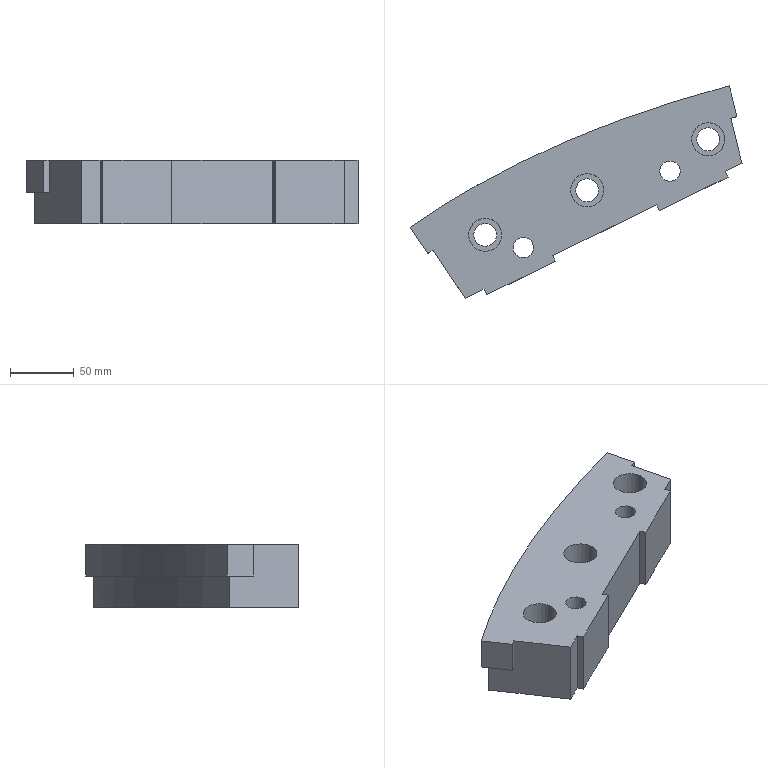Part | NX | features solid 2 | 1 solid | 31 faces | box 260.567 x 166.598 x 50 mm | volume 838150 mm3 | plane 19 | cylinder 8 | spline 4 | commonest cylinder face diameters 18 x3 26 x3 16 x2
STEP:
#1=CARTESIAN_POINT('',(-498.047,350.703,-50.));
#2=VERTEX_POINT('',#1);
#3=CARTESIAN_POINT('',(-507.047,350.703,-50.));
#4=DIRECTION('',(0.,0.,1.));
#5=DIRECTION('',(1.,0.,0.));
#6=AXIS2_PLACEMENT_3D('',#3,#4,#5);
#7=CIRCLE('',#6,9.);
#8=EDGE_CURVE('',#2,#2,#7,.T.);
#9=ORIENTED_EDGE('',*,*,#8,.T.);
#10=EDGE_LOOP('',(#9));
#11=FACE_BOUND('',#10,.T.);
#12=CARTESIAN_POINT('',(-469.047,340.703,-50.));
#13=VERTEX_POINT('',#12);
#14=CARTESIAN_POINT('',(-477.047,340.703,-50.));
#15=DIRECTION('',(0.,0.,1.));
#16=DIRECTION('',(1.,0.,0.));
#17=AXIS2_PLACEMENT_3D('',#14,#15,#16);
#18=CIRCLE('',#17,8.);
#19=EDGE_CURVE('',#13,#13,#18,.T.);
#20=ORIENTED_EDGE('',*,*,#19,.T.);
#21=EDGE_LOOP('',(#20));
#22=FACE_BOUND('',#21,.T.);
#23=CARTESIAN_POINT('',(-354.047,400.703,-50.));
#24=VERTEX_POINT('',#23);
#25=CARTESIAN_POINT('',(-362.047,400.703,-50.));
#26=DIRECTION('',(0.,0.,1.));
#27=DIRECTION('',(1.,0.,0.));
#28=AXIS2_PLACEMENT_3D('',#25,#26,#27);
#29=CIRCLE('',#28,8.);
#30=EDGE_CURVE('',#24,#24,#29,.T.);
#31=ORIENTED_EDGE('',*,*,#30,.T.);
#32=EDGE_LOOP('',(#31));
#33=FACE_BOUND('',#32,.T.);
#34=CARTESIAN_POINT('',(-323.047,425.703,-50.));
#35=VERTEX_POINT('',#34);
#36=CARTESIAN_POINT('',(-332.047,425.703,-50.));
#37=DIRECTION('',(0.,0.,1.));
#38=DIRECTION('',(1.,0.,0.));
#39=AXIS2_PLACEMENT_3D('',#36,#37,#38);
#40=CIRCLE('',#39,9.);
#41=EDGE_CURVE('',#35,#35,#40,.T.);
#42=ORIENTED_EDGE('',*,*,#41,.T.);
#43=EDGE_LOOP('',(#42));
#44=FACE_BOUND('',#43,.T.);
#45=CARTESIAN_POINT('',(-522.586,301.062,-50.));
#46=VERTEX_POINT('',#45);
#47=CARTESIAN_POINT('',(-508.006,308.173,-50.));
#48=VERTEX_POINT('',#47);
#49=CARTESIAN_POINT('',(-578.443,273.819,-50.));
#50=DIRECTION('',(0.8988,0.4384,0.));
#51=VECTOR('',#50,1000.);
#52=LINE('',#49,#51);
#53=EDGE_CURVE('',#46,#48,#52,.T.);
#54=ORIENTED_EDGE('',*,*,#53,.F.);
#55=CARTESIAN_POINT('',(-559.181,355.316,-50.));
#56=VERTEX_POINT('',#55);
#57=CARTESIAN_POINT('',(158.716,-709.011,-50.));
#58=DIRECTION('',(-0.5592,0.829,0.));
#59=VECTOR('',#58,1000.);
#60=LINE('',#57,#59);
#61=EDGE_CURVE('',#46,#56,#60,.T.);
#62=ORIENTED_EDGE('',*,*,#61,.T.);
#63=CARTESIAN_POINT('',(-319.133,461.526,-50.));
#64=VERTEX_POINT('',#63);
#65=CARTESIAN_POINT('',(-559.181,355.316,-50.));
#66=CARTESIAN_POINT('',(-554.765,358.346,-50.));
#67=CARTESIAN_POINT('',(-545.797,364.324,-50.));
#68=CARTESIAN_POINT('',(-531.933,373.042,-50.));
#69=CARTESIAN_POINT('',(-520.049,380.094,-50.));
#70=CARTESIAN_POINT('',(-511.534,384.931,-50.));
#71=CARTESIAN_POINT('',(-506.645,387.648,-50.));
#72=CARTESIAN_POINT('',(-502.873,389.713,-50.));
#73=CARTESIAN_POINT('',(-499.379,391.6,-50.));
#74=CARTESIAN_POINT('',(-494.59,394.15,-50.));
#75=CARTESIAN_POINT('',(-486.188,398.533,-50.));
#76=CARTESIAN_POINT('',(-473.957,404.65,-50.));
#77=CARTESIAN_POINT('',(-461.477,410.549,-50.));
#78=CARTESIAN_POINT('',(-452.581,414.577,-50.));
#79=CARTESIAN_POINT('',(-447.486,416.835,-50.));
#80=CARTESIAN_POINT('',(-443.565,418.547,-50.));
#81=CARTESIAN_POINT('',(-439.928,420.112,-50.));
#82=CARTESIAN_POINT('',(-434.948,422.227,-50.));
#83=CARTESIAN_POINT('',(-426.215,425.856,-50.));
#84=CARTESIAN_POINT('',(-413.532,430.907,-50.));
#85=CARTESIAN_POINT('',(-400.591,435.769,-50.));
#86=CARTESIAN_POINT('',(-390.125,439.533,-50.));
#87=CARTESIAN_POINT('',(-382.095,442.334,-50.));
#88=CARTESIAN_POINT('',(-374.392,444.943,-50.));
#89=CARTESIAN_POINT('',(-363.96,448.377,-50.));
#90=CARTESIAN_POINT('',(-345.662,454.133,-50.));
#91=CARTESIAN_POINT('',(-329.787,458.676,-50.));
#92=CARTESIAN_POINT('',(-319.133,461.526,-50.));
#93=B_SPLINE_CURVE_WITH_KNOTS('',3,(#65,#66,#67,#68,#69,#70,#71,#72,#73,#74,#75,#76,#77,#78,#79,#80,#81,#82,#83,#84,#85,#86,#87,#88,#89,#90,#91,#92),.UNSPECIFIED.,.F.,.F.,(4,1,1,1,1,1,1,1,1,1,1,1,1,1,1,1,1,1,1,1,1,1,1,1,1,4),(0.,0.0625,0.125,0.1875,0.2188,0.2344,0.25,0.2656,0.2812,0.3125,0.375,0.4375,0.4688,0.4844,0.5,0.5156,0.5312,0.5625,0.625,0.6875,0.7188,0.75,0.7812,0.8125,0.875,1.),.UNSPECIFIED.);
#94=EDGE_CURVE('',#56,#64,#93,.T.);
#95=ORIENTED_EDGE('',*,*,#94,.T.);
#96=CARTESIAN_POINT('',(-305.521,406.931,-50.));
#97=VERTEX_POINT('',#96);
#98=CARTESIAN_POINT('',(2.961,-830.323,-50.));
#99=DIRECTION('',(-0.2419,0.9703,0.));
#100=VECTOR('',#99,1000.);
#101=LINE('',#98,#100);
#102=EDGE_CURVE('',#97,#64,#101,.T.);
#103=ORIENTED_EDGE('',*,*,#102,.F.);
#104=CARTESIAN_POINT('',(-318.612,400.547,-50.));
#105=VERTEX_POINT('',#104);
#106=CARTESIAN_POINT('',(-578.443,273.819,-50.));
#107=DIRECTION('',(0.8988,0.4384,0.));
#108=VECTOR('',#107,1000.);
#109=LINE('',#106,#108);
#110=EDGE_CURVE('',#105,#97,#109,.T.);
#111=ORIENTED_EDGE('',*,*,#110,.F.);
#112=CARTESIAN_POINT('',(-316.42,396.053,-50.));
#113=VERTEX_POINT('',#112);
#114=CARTESIAN_POINT('',(-309.844,382.571,-50.));
#115=DIRECTION('',(0.4384,-0.8988,0.));
#116=VECTOR('',#115,1000.);
#117=LINE('',#114,#116);
#118=EDGE_CURVE('',#105,#113,#117,.T.);
#119=ORIENTED_EDGE('',*,*,#118,.T.);
#120=CARTESIAN_POINT('',(-370.348,369.75,-50.));
#121=VERTEX_POINT('',#120);
#122=CARTESIAN_POINT('',(-576.251,269.325,-50.));
#123=DIRECTION('',(0.8988,0.4384,0.));
#124=VECTOR('',#123,1000.);
#125=LINE('',#122,#124);
#126=EDGE_CURVE('',#121,#113,#125,.T.);
#127=ORIENTED_EDGE('',*,*,#126,.F.);
#128=CARTESIAN_POINT('',(-372.54,374.244,-50.));
#129=VERTEX_POINT('',#128);
#130=CARTESIAN_POINT('',(-363.772,356.268,-50.));
#131=DIRECTION('',(0.4384,-0.8988,0.));
#132=VECTOR('',#131,1000.);
#133=LINE('',#130,#132);
#134=EDGE_CURVE('',#129,#121,#133,.T.);
#135=ORIENTED_EDGE('',*,*,#134,.F.);
#136=CARTESIAN_POINT('',(-454.078,334.475,-50.));
#137=VERTEX_POINT('',#136);
#138=CARTESIAN_POINT('',(-578.443,273.819,-50.));
#139=DIRECTION('',(0.8988,0.4384,0.));
#140=VECTOR('',#139,1000.);
#141=LINE('',#138,#140);
#142=EDGE_CURVE('',#137,#129,#141,.T.);
#143=ORIENTED_EDGE('',*,*,#142,.F.);
#144=CARTESIAN_POINT('',(-451.886,329.981,-50.));
#145=VERTEX_POINT('',#144);
#146=CARTESIAN_POINT('',(-445.311,316.499,-50.));
#147=DIRECTION('',(0.4384,-0.8988,0.));
#148=VECTOR('',#147,1000.);
#149=LINE('',#146,#148);
#150=EDGE_CURVE('',#137,#145,#149,.T.);
#151=ORIENTED_EDGE('',*,*,#150,.T.);
#152=CARTESIAN_POINT('',(-505.814,303.679,-50.));
#153=VERTEX_POINT('',#152);
#154=CARTESIAN_POINT('',(-576.251,269.325,-50.));
#155=DIRECTION('',(0.8988,0.4384,0.));
#156=VECTOR('',#155,1000.);
#157=LINE('',#154,#156);
#158=EDGE_CURVE('',#153,#145,#157,.T.);
#159=ORIENTED_EDGE('',*,*,#158,.F.);
#160=CARTESIAN_POINT('',(-499.239,290.197,-50.));
#161=DIRECTION('',(0.4384,-0.8988,0.));
#162=VECTOR('',#161,1000.);
#163=LINE('',#160,#162);
#164=EDGE_CURVE('',#48,#153,#163,.T.);
#165=ORIENTED_EDGE('',*,*,#164,.F.);
#166=EDGE_LOOP('',(#54,#62,#95,#103,#111,#119,#127,#135,#143,#151,#159,#165));
#167=FACE_BOUND('',#166,.T.);
#168=CARTESIAN_POINT('',(-418.047,385.703,-50.));
#169=VERTEX_POINT('',#168);
#170=CARTESIAN_POINT('',(-427.047,385.703,-50.));
#171=DIRECTION('',(0.,0.,1.));
#172=DIRECTION('',(1.,0.,0.));
#173=AXIS2_PLACEMENT_3D('',#170,#171,#172);
#174=CIRCLE('',#173,9.);
#175=EDGE_CURVE('',#169,#169,#174,.F.);
#176=ORIENTED_EDGE('',*,*,#175,.F.);
#177=EDGE_LOOP('',(#176));
#178=FACE_BOUND('',#177,.T.);
#179=CARTESIAN_POINT('',(-35.268,-839.855,-50.));
#180=DIRECTION('',(0.,0.,1.));
#181=DIRECTION('',(1.,0.,0.));
#182=AXIS2_PLACEMENT_3D('',#179,#180,#181);
#183=PLANE('',#182);
#184=ADVANCED_FACE('',(#11,#22,#33,#44,#167,#178),#183,.F.);
#185=CARTESIAN_POINT('',(-414.047,385.703,-30.));
#186=VERTEX_POINT('',#185);
#187=CARTESIAN_POINT('',(-427.047,385.703,-30.));
#188=DIRECTION('',(0.,0.,1.));
#189=DIRECTION('',(1.,0.,0.));
#190=AXIS2_PLACEMENT_3D('',#187,#188,#189);
#191=CIRCLE('',#190,13.);
#192=EDGE_CURVE('',#186,#186,#191,.T.);
#193=ORIENTED_EDGE('',*,*,#192,.T.);
#194=EDGE_LOOP('',(#193));
#195=FACE_BOUND('',#194,.T.);
#196=CARTESIAN_POINT('',(-418.047,385.703,-30.));
#197=VERTEX_POINT('',#196);
#198=CARTESIAN_POINT('',(-427.047,385.703,-30.));
#199=DIRECTION('',(0.,0.,1.));
#200=DIRECTION('',(1.,0.,0.));
#201=AXIS2_PLACEMENT_3D('',#198,#199,#200);
#202=CIRCLE('',#201,9.);
#203=EDGE_CURVE('',#197,#197,#202,.F.);
#204=ORIENTED_EDGE('',*,*,#203,.T.);
#205=EDGE_LOOP('',(#204));
#206=FACE_BOUND('',#205,.T.);
#207=CARTESIAN_POINT('',(-427.047,385.703,-30.));
#208=DIRECTION('',(0.,0.,1.));
#209=DIRECTION('',(1.,0.,0.));
#210=AXIS2_PLACEMENT_3D('',#207,#208,#209);
#211=PLANE('',#210);
#212=ADVANCED_FACE('',(#195,#206),#211,.T.);
#213=CARTESIAN_POINT('',(-354.047,400.703,0.));
#214=VERTEX_POINT('',#213);
#215=CARTESIAN_POINT('',(-362.047,400.703,0.));
#216=DIRECTION('',(0.,0.,1.));
#217=DIRECTION('',(1.,0.,0.));
#218=AXIS2_PLACEMENT_3D('',#215,#216,#217);
#219=CIRCLE('',#218,8.);
#220=EDGE_CURVE('',#214,#214,#219,.T.);
#221=ORIENTED_EDGE('',*,*,#220,.F.);
#222=EDGE_LOOP('',(#221));
#223=FACE_BOUND('',#222,.T.);
#224=CARTESIAN_POINT('',(-469.047,340.703,0.));
#225=VERTEX_POINT('',#224);
#226=CARTESIAN_POINT('',(-477.047,340.703,0.));
#227=DIRECTION('',(0.,0.,1.));
#228=DIRECTION('',(1.,0.,0.));
#229=AXIS2_PLACEMENT_3D('',#226,#227,#228);
#230=CIRCLE('',#229,8.);
#231=EDGE_CURVE('',#225,#225,#230,.T.);
#232=ORIENTED_EDGE('',*,*,#231,.F.);
#233=EDGE_LOOP('',(#232));
#234=FACE_BOUND('',#233,.T.);
#235=CARTESIAN_POINT('',(-319.047,425.703,0.));
#236=VERTEX_POINT('',#235);
#237=CARTESIAN_POINT('',(-332.047,425.703,0.));
#238=DIRECTION('',(0.,0.,1.));
#239=DIRECTION('',(1.,0.,0.));
#240=AXIS2_PLACEMENT_3D('',#237,#238,#239);
#241=CIRCLE('',#240,13.);
#242=EDGE_CURVE('',#236,#236,#241,.T.);
#243=ORIENTED_EDGE('',*,*,#242,.F.);
#244=EDGE_LOOP('',(#243));
#245=FACE_BOUND('',#244,.T.);
#246=CARTESIAN_POINT('',(-494.047,350.703,0.));
#247=VERTEX_POINT('',#246);
#248=CARTESIAN_POINT('',(-507.047,350.703,0.));
#249=DIRECTION('',(0.,0.,1.));
#250=DIRECTION('',(1.,0.,0.));
#251=AXIS2_PLACEMENT_3D('',#248,#249,#250);
#252=CIRCLE('',#251,13.);
#253=EDGE_CURVE('',#247,#247,#252,.T.);
#254=ORIENTED_EDGE('',*,*,#253,.F.);
#255=EDGE_LOOP('',(#254));
#256=FACE_BOUND('',#255,.T.);
#257=CARTESIAN_POINT('',(-552.106,335.886,0.));
#258=VERTEX_POINT('',#257);
#259=CARTESIAN_POINT('',(-566.088,356.614,0.));
#260=VERTEX_POINT('',#259);
#261=CARTESIAN_POINT('',(-500.019,258.663,0.));
#262=DIRECTION('',(-0.5592,0.829,0.));
#263=VECTOR('',#262,1000.);
#264=LINE('',#261,#263);
#265=EDGE_CURVE('',#258,#260,#264,.T.);
#266=ORIENTED_EDGE('',*,*,#265,.F.);
#267=CARTESIAN_POINT('',(-547.997,338.734,0.));
#268=VERTEX_POINT('',#267);
#269=CARTESIAN_POINT('',(-547.997,338.734,0.));
#270=CARTESIAN_POINT('',(-549.371,337.791,0.));
#271=CARTESIAN_POINT('',(-550.74,336.84,0.));
#272=CARTESIAN_POINT('',(-552.106,335.886,0.));
#273=B_SPLINE_CURVE_WITH_KNOTS('',3,(#269,#270,#271,#272),.UNSPECIFIED.,.F.,.F.,(4,4),(0.5979,0.6029),.UNSPECIFIED.);
#274=EDGE_CURVE('',#258,#268,#273,.F.);
#275=ORIENTED_EDGE('',*,*,#274,.T.);
#276=CARTESIAN_POINT('',(-522.586,301.062,0.));
#277=VERTEX_POINT('',#276);
#278=CARTESIAN_POINT('',(-497.568,263.971,0.));
#279=DIRECTION('',(0.5592,-0.829,0.));
#280=VECTOR('',#279,1000.);
#281=LINE('',#278,#280);
#282=EDGE_CURVE('',#268,#277,#281,.T.);
#283=ORIENTED_EDGE('',*,*,#282,.T.);
#284=CARTESIAN_POINT('',(-508.006,308.173,0.));
#285=VERTEX_POINT('',#284);
#286=CARTESIAN_POINT('',(-521.061,301.806,0.));
#287=DIRECTION('',(-0.8988,-0.4384,0.));
#288=VECTOR('',#287,1000.);
#289=LINE('',#286,#288);
#290=EDGE_CURVE('',#285,#277,#289,.T.);
#291=ORIENTED_EDGE('',*,*,#290,.F.);
#292=CARTESIAN_POINT('',(-505.814,303.679,0.));
#293=VERTEX_POINT('',#292);
#294=CARTESIAN_POINT('',(-538.254,370.19,0.));
#295=DIRECTION('',(0.4384,-0.8988,0.));
#296=VECTOR('',#295,1000.);
#297=LINE('',#294,#296);
#298=EDGE_CURVE('',#285,#293,#297,.T.);
#299=ORIENTED_EDGE('',*,*,#298,.T.);
#300=CARTESIAN_POINT('',(-451.886,329.981,0.));
#301=VERTEX_POINT('',#300);
#302=CARTESIAN_POINT('',(-518.869,297.312,0.));
#303=DIRECTION('',(0.8988,0.4384,0.));
#304=VECTOR('',#303,1000.);
#305=LINE('',#302,#304);
#306=EDGE_CURVE('',#293,#301,#305,.T.);
#307=ORIENTED_EDGE('',*,*,#306,.T.);
#308=CARTESIAN_POINT('',(-454.078,334.475,0.));
#309=VERTEX_POINT('',#308);
#310=CARTESIAN_POINT('',(-484.326,396.492,0.));
#311=DIRECTION('',(0.4384,-0.8988,0.));
#312=VECTOR('',#311,1000.);
#313=LINE('',#310,#312);
#314=EDGE_CURVE('',#309,#301,#313,.T.);
#315=ORIENTED_EDGE('',*,*,#314,.F.);
#316=CARTESIAN_POINT('',(-372.54,374.244,0.));
#317=VERTEX_POINT('',#316);
#318=CARTESIAN_POINT('',(-521.061,301.806,0.));
#319=DIRECTION('',(-0.8988,-0.4384,0.));
#320=VECTOR('',#319,1000.);
#321=LINE('',#318,#320);
#322=EDGE_CURVE('',#317,#309,#321,.T.);
#323=ORIENTED_EDGE('',*,*,#322,.F.);
#324=CARTESIAN_POINT('',(-370.348,369.75,0.));
#325=VERTEX_POINT('',#324);
#326=CARTESIAN_POINT('',(-402.787,436.261,0.));
#327=DIRECTION('',(0.4384,-0.8988,0.));
#328=VECTOR('',#327,1000.);
#329=LINE('',#326,#328);
#330=EDGE_CURVE('',#317,#325,#329,.T.);
#331=ORIENTED_EDGE('',*,*,#330,.T.);
#332=CARTESIAN_POINT('',(-316.42,396.053,0.));
#333=VERTEX_POINT('',#332);
#334=CARTESIAN_POINT('',(-518.869,297.312,0.));
#335=DIRECTION('',(0.8988,0.4384,0.));
#336=VECTOR('',#335,1000.);
#337=LINE('',#334,#336);
#338=EDGE_CURVE('',#325,#333,#337,.T.);
#339=ORIENTED_EDGE('',*,*,#338,.T.);
#340=CARTESIAN_POINT('',(-318.612,400.547,0.));
#341=VERTEX_POINT('',#340);
#342=CARTESIAN_POINT('',(-348.86,462.564,0.));
#343=DIRECTION('',(0.4384,-0.8988,0.));
#344=VECTOR('',#343,1000.);
#345=LINE('',#342,#344);
#346=EDGE_CURVE('',#341,#333,#345,.T.);
#347=ORIENTED_EDGE('',*,*,#346,.F.);
#348=CARTESIAN_POINT('',(-305.521,406.931,0.));
#349=VERTEX_POINT('',#348);
#350=CARTESIAN_POINT('',(-521.061,301.806,0.));
#351=DIRECTION('',(-0.8988,-0.4384,0.));
#352=VECTOR('',#351,1000.);
#353=LINE('',#350,#352);
#354=EDGE_CURVE('',#349,#341,#353,.T.);
#355=ORIENTED_EDGE('',*,*,#354,.F.);
#356=CARTESIAN_POINT('',(-314.294,442.117,0.));
#357=VERTEX_POINT('',#356);
#358=CARTESIAN_POINT('',(-294.648,363.324,0.));
#359=DIRECTION('',(0.2419,-0.9703,0.));
#360=VECTOR('',#359,1000.);
#361=LINE('',#358,#360);
#362=EDGE_CURVE('',#357,#349,#361,.T.);
#363=ORIENTED_EDGE('',*,*,#362,.F.);
#364=CARTESIAN_POINT('',(-309.461,443.4,0.));
#365=VERTEX_POINT('',#364);
#366=CARTESIAN_POINT('',(-309.461,443.4,0.));
#367=CARTESIAN_POINT('',(-311.073,442.976,0.));
#368=CARTESIAN_POINT('',(-312.684,442.548,0.));
#369=CARTESIAN_POINT('',(-314.294,442.117,0.));
#370=B_SPLINE_CURVE_WITH_KNOTS('',3,(#366,#367,#368,#369),.UNSPECIFIED.,.F.,.F.,(4,4),(0.3359,0.3409),.UNSPECIFIED.);
#371=EDGE_CURVE('',#357,#365,#370,.F.);
#372=ORIENTED_EDGE('',*,*,#371,.T.);
#373=CARTESIAN_POINT('',(-315.509,467.66,0.));
#374=VERTEX_POINT('',#373);
#375=CARTESIAN_POINT('',(-277.249,314.206,0.));
#376=DIRECTION('',(-0.2419,0.9703,0.));
#377=VECTOR('',#376,1000.);
#378=LINE('',#375,#377);
#379=EDGE_CURVE('',#365,#374,#378,.T.);
#380=ORIENTED_EDGE('',*,*,#379,.T.);
#381=CARTESIAN_POINT('',(-315.509,467.66,0.));
#382=CARTESIAN_POINT('',(-337.712,461.819,0.));
#383=CARTESIAN_POINT('',(-370.715,451.94,0.));
#384=CARTESIAN_POINT('',(-414.062,436.257,0.));
#385=CARTESIAN_POINT('',(-456.885,418.756,0.));
#386=CARTESIAN_POINT('',(-508.381,393.676,0.));
#387=CARTESIAN_POINT('',(-547.311,369.734,0.));
#388=CARTESIAN_POINT('',(-566.088,356.614,0.));
#389=B_SPLINE_CURVE_WITH_KNOTS('',3,(#381,#382,#383,#384,#385,#386,#387,#388),.UNSPECIFIED.,.F.,.F.,(4,1,1,1,1,4),(0.7591,0.828,0.8624,0.8968,0.9657,1.035),.UNSPECIFIED.);
#390=EDGE_CURVE('',#260,#374,#389,.F.);
#391=ORIENTED_EDGE('',*,*,#390,.F.);
#392=EDGE_LOOP('',(#266,#275,#283,#291,#299,#307,#315,#323,#331,#339,#347,#355,#363,#372,#380,#391));
#393=FACE_BOUND('',#392,.T.);
#394=CARTESIAN_POINT('',(-414.047,385.703,0.));
#395=VERTEX_POINT('',#394);
#396=CARTESIAN_POINT('',(-427.047,385.703,0.));
#397=DIRECTION('',(0.,0.,1.));
#398=DIRECTION('',(1.,0.,0.));
#399=AXIS2_PLACEMENT_3D('',#396,#397,#398);
#400=CIRCLE('',#399,13.);
#401=EDGE_CURVE('',#395,#395,#400,.F.);
#402=ORIENTED_EDGE('',*,*,#401,.T.);
#403=EDGE_LOOP('',(#402));
#404=FACE_BOUND('',#403,.T.);
#405=CARTESIAN_POINT('',(-500.019,258.663,0.));
#406=DIRECTION('',(0.,0.,1.));
#407=DIRECTION('',(1.,0.,0.));
#408=AXIS2_PLACEMENT_3D('',#405,#406,#407);
#409=PLANE('',#408);
#410=ADVANCED_FACE('',(#223,#234,#245,#256,#393,#404),#409,.T.);
#411=CARTESIAN_POINT('',(-547.997,338.734,-25.));
#412=VERTEX_POINT('',#411);
#413=CARTESIAN_POINT('',(-547.997,338.734,-25.));
#414=DIRECTION('',(0.,0.,-1.));
#415=VECTOR('',#414,1000.);
#416=LINE('',#413,#415);
#417=EDGE_CURVE('',#412,#268,#416,.F.);
#418=ORIENTED_EDGE('',*,*,#417,.T.);
#419=ORIENTED_EDGE('',*,*,#274,.F.);
#420=CARTESIAN_POINT('',(-552.106,335.886,-25.));
#421=VERTEX_POINT('',#420);
#422=CARTESIAN_POINT('',(-552.106,335.886,0.));
#423=DIRECTION('',(0.,0.,-1.));
#424=VECTOR('',#423,1000.);
#425=LINE('',#422,#424);
#426=EDGE_CURVE('',#258,#421,#425,.T.);
#427=ORIENTED_EDGE('',*,*,#426,.T.);
#428=CARTESIAN_POINT('',(-552.106,335.886,-25.));
#429=CARTESIAN_POINT('',(-550.685,336.879,-25.));
#430=CARTESIAN_POINT('',(-549.366,337.794,-25.));
#431=CARTESIAN_POINT('',(-547.997,338.734,-25.));
#432=B_SPLINE_CURVE_WITH_KNOTS('',3,(#428,#429,#430,#431),.UNSPECIFIED.,.F.,.F.,(4,4),(-0.001492,0.01739),.UNSPECIFIED.);
#433=EDGE_CURVE('',#421,#412,#432,.T.);
#434=ORIENTED_EDGE('',*,*,#433,.T.);
#435=EDGE_LOOP('',(#418,#419,#427,#434));
#436=FACE_BOUND('',#435,.T.);
#437=CARTESIAN_POINT('',(-552.106,335.886,0.));
#438=CARTESIAN_POINT('',(-552.106,335.886,-25.));
#439=CARTESIAN_POINT('',(-550.685,336.879,0.));
#440=CARTESIAN_POINT('',(-550.685,336.879,-25.));
#441=CARTESIAN_POINT('',(-549.366,337.794,0.));
#442=CARTESIAN_POINT('',(-549.366,337.794,-25.));
#443=CARTESIAN_POINT('',(-547.997,338.734,0.));
#444=CARTESIAN_POINT('',(-547.997,338.734,-25.));
#445=B_SPLINE_SURFACE_WITH_KNOTS('',3,1,((#437,#438),(#439,#440),(#441,#442),(#443,#444)),.SURF_OF_LINEAR_EXTRUSION.,.F.,.F.,.F.,(4,4),(2,2),(-0.001492,0.01739),(0.,1.),.PIECEWISE_BEZIER_KNOTS.);
#446=ADVANCED_FACE('',(#436),#445,.F.);
#447=ORIENTED_EDGE('',*,*,#8,.F.);
#448=EDGE_LOOP('',(#447));
#449=FACE_BOUND('',#448,.T.);
#450=CARTESIAN_POINT('',(-498.047,350.703,-30.));
#451=VERTEX_POINT('',#450);
#452=CARTESIAN_POINT('',(-507.047,350.703,-30.));
#453=DIRECTION('',(0.,0.,1.));
#454=DIRECTION('',(1.,0.,0.));
#455=AXIS2_PLACEMENT_3D('',#452,#453,#454);
#456=CIRCLE('',#455,9.);
#457=EDGE_CURVE('',#451,#451,#456,.F.);
#458=ORIENTED_EDGE('',*,*,#457,.F.);
#459=EDGE_LOOP('',(#458));
#460=FACE_BOUND('',#459,.T.);
#461=CARTESIAN_POINT('',(-507.047,350.703,-125.));
#462=DIRECTION('',(0.,0.,1.));
#463=DIRECTION('',(1.,0.,0.));
#464=AXIS2_PLACEMENT_3D('',#461,#462,#463);
#465=CYLINDRICAL_SURFACE('',#464,9.);
#466=ADVANCED_FACE('',(#449,#460),#465,.F.);
#467=ORIENTED_EDGE('',*,*,#41,.F.);
#468=EDGE_LOOP('',(#467));
#469=FACE_BOUND('',#468,.T.);
#470=CARTESIAN_POINT('',(-323.047,425.703,-30.));
#471=VERTEX_POINT('',#470);
#472=CARTESIAN_POINT('',(-332.047,425.703,-30.));
#473=DIRECTION('',(0.,0.,1.));
#474=DIRECTION('',(1.,0.,0.));
#475=AXIS2_PLACEMENT_3D('',#472,#473,#474);
#476=CIRCLE('',#475,9.);
#477=EDGE_CURVE('',#471,#471,#476,.F.);
#478=ORIENTED_EDGE('',*,*,#477,.F.);
#479=EDGE_LOOP('',(#478));
#480=FACE_BOUND('',#479,.T.);
#481=CARTESIAN_POINT('',(-332.047,425.703,-125.));
#482=DIRECTION('',(0.,0.,1.));
#483=DIRECTION('',(1.,0.,0.));
#484=AXIS2_PLACEMENT_3D('',#481,#482,#483);
#485=CYLINDRICAL_SURFACE('',#484,9.);
#486=ADVANCED_FACE('',(#469,#480),#485,.F.);
#487=ORIENTED_EDGE('',*,*,#354,.T.);
#488=CARTESIAN_POINT('',(-318.612,400.547,-70.));
#489=DIRECTION('',(0.,0.,-1.));
#490=VECTOR('',#489,1000.);
#491=LINE('',#488,#490);
#492=EDGE_CURVE('',#341,#105,#491,.T.);
#493=ORIENTED_EDGE('',*,*,#492,.T.);
#494=ORIENTED_EDGE('',*,*,#110,.T.);
#495=CARTESIAN_POINT('',(-305.521,406.931,-70.));
#496=DIRECTION('',(0.,0.,1.));
#497=VECTOR('',#496,1000.);
#498=LINE('',#495,#497);
#499=EDGE_CURVE('',#97,#349,#498,.T.);
#500=ORIENTED_EDGE('',*,*,#499,.T.);
#501=EDGE_LOOP('',(#487,#493,#494,#500));
#502=FACE_BOUND('',#501,.T.);
#503=CARTESIAN_POINT('',(-521.061,301.806,-70.));
#504=DIRECTION('',(0.4384,-0.8988,0.));
#505=DIRECTION('',(0.8988,0.4384,0.));
#506=AXIS2_PLACEMENT_3D('',#503,#504,#505);
#507=PLANE('',#506);
#508=ADVANCED_FACE('',(#502),#507,.T.);
#509=CARTESIAN_POINT('',(-372.54,374.244,-70.));
#510=DIRECTION('',(0.,0.,-1.));
#511=VECTOR('',#510,1000.);
#512=LINE('',#509,#511);
#513=EDGE_CURVE('',#317,#129,#512,.T.);
#514=ORIENTED_EDGE('',*,*,#513,.F.);
#515=ORIENTED_EDGE('',*,*,#322,.T.);
#516=CARTESIAN_POINT('',(-454.078,334.475,-70.));
#517=DIRECTION('',(0.,0.,-1.));
#518=VECTOR('',#517,1000.);
#519=LINE('',#516,#518);
#520=EDGE_CURVE('',#309,#137,#519,.T.);
#521=ORIENTED_EDGE('',*,*,#520,.T.);
#522=ORIENTED_EDGE('',*,*,#142,.T.);
#523=EDGE_LOOP('',(#514,#515,#521,#522));
#524=FACE_BOUND('',#523,.T.);
#525=CARTESIAN_POINT('',(-521.061,301.806,-70.));
#526=DIRECTION('',(0.4384,-0.8988,0.));
#527=DIRECTION('',(0.8988,0.4384,0.));
#528=AXIS2_PLACEMENT_3D('',#525,#526,#527);
#529=PLANE('',#528);
#530=ADVANCED_FACE('',(#524),#529,.T.);
#531=CARTESIAN_POINT('',(-508.006,308.173,-70.));
#532=DIRECTION('',(0.,0.,-1.));
#533=VECTOR('',#532,1000.);
#534=LINE('',#531,#533);
#535=EDGE_CURVE('',#285,#48,#534,.T.);
#536=ORIENTED_EDGE('',*,*,#535,.F.);
#537=ORIENTED_EDGE('',*,*,#290,.T.);
#538=CARTESIAN_POINT('',(-522.586,301.062,-70.));
#539=DIRECTION('',(0.,0.,1.));
#540=VECTOR('',#539,1000.);
#541=LINE('',#538,#540);
#542=EDGE_CURVE('',#46,#277,#541,.T.);
#543=ORIENTED_EDGE('',*,*,#542,.F.);
#544=ORIENTED_EDGE('',*,*,#53,.T.);
#545=EDGE_LOOP('',(#536,#537,#543,#544));
#546=FACE_BOUND('',#545,.T.);
#547=CARTESIAN_POINT('',(-521.061,301.806,-70.));
#548=DIRECTION('',(0.4384,-0.8988,0.));
#549=DIRECTION('',(0.8988,0.4384,0.));
#550=AXIS2_PLACEMENT_3D('',#547,#548,#549);
#551=PLANE('',#550);
#552=ADVANCED_FACE('',(#546),#551,.T.);
#553=ORIENTED_EDGE('',*,*,#433,.F.);
#554=CARTESIAN_POINT('',(-566.088,356.614,-25.));
#555=VERTEX_POINT('',#554);
#556=CARTESIAN_POINT('',(-566.088,356.614,-25.));
#557=DIRECTION('',(0.5592,-0.829,0.));
#558=VECTOR('',#557,1000.);
#559=LINE('',#556,#558);
#560=EDGE_CURVE('',#555,#421,#559,.T.);
#561=ORIENTED_EDGE('',*,*,#560,.F.);
#562=CARTESIAN_POINT('',(-315.509,467.66,-25.));
#563=VERTEX_POINT('',#562);
#564=CARTESIAN_POINT('',(-315.509,467.66,-25.));
#565=CARTESIAN_POINT('',(-337.671,461.83,-25.));
#566=CARTESIAN_POINT('',(-370.615,451.97,-25.));
#567=CARTESIAN_POINT('',(-413.838,436.341,-25.));
#568=CARTESIAN_POINT('',(-445.942,423.238,-25.));
#569=CARTESIAN_POINT('',(-477.424,408.749,-25.));
#570=CARTESIAN_POINT('',(-518.165,387.668,-25.));
#571=CARTESIAN_POINT('',(-547.353,369.704,-25.));
#572=CARTESIAN_POINT('',(-566.088,356.614,-25.));
#573=B_SPLINE_CURVE_WITH_KNOTS('',3,(#564,#565,#566,#567,#568,#569,#570,#571,#572),.UNSPECIFIED.,.F.,.F.,(4,1,1,1,1,1,4),(0.7372,0.806,0.8404,0.8747,0.9091,0.9435,1.012),.UNSPECIFIED.);
#574=EDGE_CURVE('',#555,#563,#573,.F.);
#575=ORIENTED_EDGE('',*,*,#574,.T.);
#576=CARTESIAN_POINT('',(-309.461,443.4,-25.));
#577=VERTEX_POINT('',#576);
#578=CARTESIAN_POINT('',(296.577,-1987.282,-25.));
#579=DIRECTION('',(-0.2419,0.9703,0.));
#580=VECTOR('',#579,1000.);
#581=LINE('',#578,#580);
#582=EDGE_CURVE('',#577,#563,#581,.T.);
#583=ORIENTED_EDGE('',*,*,#582,.F.);
#584=CARTESIAN_POINT('',(-314.294,442.117,-25.));
#585=VERTEX_POINT('',#584);
#586=CARTESIAN_POINT('',(-314.294,442.117,-25.));
#587=CARTESIAN_POINT('',(-312.687,442.547,-25.));
#588=CARTESIAN_POINT('',(-311.076,442.975,-25.));
#589=CARTESIAN_POINT('',(-309.461,443.4,-25.));
#590=B_SPLINE_CURVE_WITH_KNOTS('',3,(#586,#587,#588,#589),.UNSPECIFIED.,.F.,.F.,(4,4),(0.9803,0.9988),.UNSPECIFIED.);
#591=EDGE_CURVE('',#585,#577,#590,.T.);
#592=ORIENTED_EDGE('',*,*,#591,.F.);
#593=CARTESIAN_POINT('',(-319.133,461.526,-25.));
#594=VERTEX_POINT('',#593);
#595=CARTESIAN_POINT('',(-294.648,363.324,-25.));
#596=DIRECTION('',(-0.2419,0.9703,0.));
#597=VECTOR('',#596,1000.);
#598=LINE('',#595,#597);
#599=EDGE_CURVE('',#585,#594,#598,.T.);
#600=ORIENTED_EDGE('',*,*,#599,.T.);
#601=CARTESIAN_POINT('',(-559.181,355.316,-25.));
#602=VERTEX_POINT('',#601);
#603=CARTESIAN_POINT('',(-559.181,355.316,-25.));
#604=CARTESIAN_POINT('',(-541.017,367.781,-25.));
#605=CARTESIAN_POINT('',(-503.487,390.554,-25.));
#606=CARTESIAN_POINT('',(-444.166,419.285,-25.));
#607=CARTESIAN_POINT('',(-382.493,443.019,-25.));
#608=CARTESIAN_POINT('',(-340.389,455.84,-25.));
#609=CARTESIAN_POINT('',(-319.133,461.526,-25.));
#610=B_SPLINE_CURVE_WITH_KNOTS('',3,(#603,#604,#605,#606,#607,#608,#609),.UNSPECIFIED.,.F.,.F.,(4,1,1,1,4),(1.121,1.187,1.253,1.319,1.385),.UNSPECIFIED.);
#611=EDGE_CURVE('',#602,#594,#610,.T.);
#612=ORIENTED_EDGE('',*,*,#611,.F.);
#613=CARTESIAN_POINT('',(-497.568,263.971,-25.));
#614=DIRECTION('',(-0.5592,0.829,0.));
#615=VECTOR('',#614,1000.);
#616=LINE('',#613,#615);
#617=EDGE_CURVE('',#412,#602,#616,.T.);
#618=ORIENTED_EDGE('',*,*,#617,.F.);
#619=EDGE_LOOP('',(#553,#561,#575,#583,#592,#600,#612,#618));
#620=FACE_BOUND('',#619,.T.);
#621=CARTESIAN_POINT('',(-566.088,356.614,-25.));
#622=DIRECTION('',(0.,0.,-1.));
#623=DIRECTION('',(-1.,0.,0.));
#624=AXIS2_PLACEMENT_3D('',#621,#622,#623);
#625=PLANE('',#624);
#626=ADVANCED_FACE('',(#620),#625,.T.);
#627=ORIENTED_EDGE('',*,*,#499,.F.);
#628=ORIENTED_EDGE('',*,*,#102,.T.);
#629=CARTESIAN_POINT('',(-319.133,461.526,-42.5));
#630=DIRECTION('',(0.,0.,1.));
#631=VECTOR('',#630,1000.);
#632=LINE('',#629,#631);
#633=EDGE_CURVE('',#64,#594,#632,.T.);
#634=ORIENTED_EDGE('',*,*,#633,.T.);
#635=ORIENTED_EDGE('',*,*,#599,.F.);
#636=CARTESIAN_POINT('',(-314.294,442.117,-25.));
#637=DIRECTION('',(0.,0.,-1.));
#638=VECTOR('',#637,1000.);
#639=LINE('',#636,#638);
#640=EDGE_CURVE('',#585,#357,#639,.F.);
#641=ORIENTED_EDGE('',*,*,#640,.T.);
#642=ORIENTED_EDGE('',*,*,#362,.T.);
#643=EDGE_LOOP('',(#627,#628,#634,#635,#641,#642));
#644=FACE_BOUND('',#643,.T.);
#645=CARTESIAN_POINT('',(-294.648,363.324,-70.));
#646=DIRECTION('',(0.9703,0.2419,0.));
#647=DIRECTION('',(-0.2419,0.9703,0.));
#648=AXIS2_PLACEMENT_3D('',#645,#646,#647);
#649=PLANE('',#648);
#650=ADVANCED_FACE('',(#644),#649,.T.);
#651=ORIENTED_EDGE('',*,*,#61,.F.);
#652=ORIENTED_EDGE('',*,*,#542,.T.);
#653=ORIENTED_EDGE('',*,*,#282,.F.);
#654=ORIENTED_EDGE('',*,*,#417,.F.);
#655=ORIENTED_EDGE('',*,*,#617,.T.);
#656=CARTESIAN_POINT('',(-559.181,355.316,-42.5));
#657=DIRECTION('',(0.,0.,1.));
#658=VECTOR('',#657,1000.);
#659=LINE('',#656,#658);
#660=EDGE_CURVE('',#56,#602,#659,.T.);
#661=ORIENTED_EDGE('',*,*,#660,.F.);
#662=EDGE_LOOP('',(#651,#652,#653,#654,#655,#661));
#663=FACE_BOUND('',#662,.T.);
#664=CARTESIAN_POINT('',(-497.568,263.971,-70.));
#665=DIRECTION('',(0.829,0.5592,0.));
#666=DIRECTION('',(-0.5592,0.829,0.));
#667=AXIS2_PLACEMENT_3D('',#664,#665,#666);
#668=PLANE('',#667);
#669=ADVANCED_FACE('',(#663),#668,.F.);
#670=ORIENTED_EDGE('',*,*,#426,.F.);
#671=ORIENTED_EDGE('',*,*,#265,.T.);
#672=CARTESIAN_POINT('',(-566.088,356.614,-70.));
#673=DIRECTION('',(0.,0.,1.));
#674=VECTOR('',#673,1000.);
#675=LINE('',#672,#674);
#676=EDGE_CURVE('',#555,#260,#675,.T.);
#677=ORIENTED_EDGE('',*,*,#676,.F.);
#678=ORIENTED_EDGE('',*,*,#560,.T.);
#679=EDGE_LOOP('',(#670,#671,#677,#678));
#680=FACE_BOUND('',#679,.T.);
#681=CARTESIAN_POINT('',(822.371,-1701.861,-70.));
#682=DIRECTION('',(0.829,0.5592,0.));
#683=DIRECTION('',(-0.5592,0.829,0.));
#684=AXIS2_PLACEMENT_3D('',#681,#682,#683);
#685=PLANE('',#684);
#686=ADVANCED_FACE('',(#680),#685,.F.);
#687=ORIENTED_EDGE('',*,*,#94,.F.);
#688=ORIENTED_EDGE('',*,*,#660,.T.);
#689=ORIENTED_EDGE('',*,*,#611,.T.);
#690=ORIENTED_EDGE('',*,*,#633,.F.);
#691=EDGE_LOOP('',(#687,#688,#689,#690));
#692=FACE_BOUND('',#691,.T.);
#693=CARTESIAN_POINT('',(-559.181,355.316,-50.));
#694=CARTESIAN_POINT('',(-559.181,355.316,-25.));
#695=CARTESIAN_POINT('',(-541.094,367.728,-50.));
#696=CARTESIAN_POINT('',(-541.094,367.728,-25.));
#697=CARTESIAN_POINT('',(-503.517,390.543,-50.));
#698=CARTESIAN_POINT('',(-503.517,390.543,-25.));
#699=CARTESIAN_POINT('',(-444.147,419.292,-50.));
#700=CARTESIAN_POINT('',(-444.147,419.292,-25.));
#701=CARTESIAN_POINT('',(-382.519,443.01,-50.));
#702=CARTESIAN_POINT('',(-382.519,443.01,-25.));
#703=CARTESIAN_POINT('',(-340.404,455.836,-50.));
#704=CARTESIAN_POINT('',(-340.404,455.836,-25.));
#705=CARTESIAN_POINT('',(-319.133,461.526,-50.));
#706=CARTESIAN_POINT('',(-319.133,461.526,-25.));
#707=B_SPLINE_SURFACE_WITH_KNOTS('',3,1,((#693,#694),(#695,#696),(#697,#698),(#699,#700),(#701,#702),(#703,#704),(#705,#706)),.SURF_OF_LINEAR_EXTRUSION.,.F.,.F.,.F.,(4,1,1,1,4),(2,2),(0.018,0.2589,0.4998,0.7407,0.9815),(0.,1.),.UNSPECIFIED.);
#708=ADVANCED_FACE('',(#692),#707,.F.);
#709=CARTESIAN_POINT('',(-309.461,443.4,-12.5));
#710=DIRECTION('',(0.,0.,-1.));
#711=VECTOR('',#710,1000.);
#712=LINE('',#709,#711);
#713=EDGE_CURVE('',#577,#365,#712,.F.);
#714=ORIENTED_EDGE('',*,*,#713,.F.);
#715=ORIENTED_EDGE('',*,*,#582,.T.);
#716=CARTESIAN_POINT('',(-315.509,467.66,-70.));
#717=DIRECTION('',(0.,0.,1.));
#718=VECTOR('',#717,1000.);
#719=LINE('',#716,#718);
#720=EDGE_CURVE('',#563,#374,#719,.T.);
#721=ORIENTED_EDGE('',*,*,#720,.T.);
#722=ORIENTED_EDGE('',*,*,#379,.F.);
#723=EDGE_LOOP('',(#714,#715,#721,#722));
#724=FACE_BOUND('',#723,.T.);
#725=CARTESIAN_POINT('',(296.577,-1987.282,-70.));
#726=DIRECTION('',(0.9703,0.2419,0.));
#727=DIRECTION('',(-0.2419,0.9703,0.));
#728=AXIS2_PLACEMENT_3D('',#725,#726,#727);
#729=PLANE('',#728);
#730=ADVANCED_FACE('',(#724),#729,.T.);
#731=ORIENTED_EDGE('',*,*,#574,.F.);
#732=ORIENTED_EDGE('',*,*,#676,.T.);
#733=ORIENTED_EDGE('',*,*,#390,.T.);
#734=ORIENTED_EDGE('',*,*,#720,.F.);
#735=EDGE_LOOP('',(#731,#732,#733,#734));
#736=FACE_BOUND('',#735,.T.);
#737=CARTESIAN_POINT('',(-566.088,356.614,-25.));
#738=CARTESIAN_POINT('',(-566.088,356.614,0.));
#739=CARTESIAN_POINT('',(-547.268,369.764,-25.));
#740=CARTESIAN_POINT('',(-547.268,369.764,0.));
#741=CARTESIAN_POINT('',(-508.094,393.851,-25.));
#742=CARTESIAN_POINT('',(-508.094,393.851,0.));
#743=CARTESIAN_POINT('',(-425.426,434.012,-25.));
#744=CARTESIAN_POINT('',(-425.426,434.012,0.));
#745=CARTESIAN_POINT('',(-359.912,455.978,-25.));
#746=CARTESIAN_POINT('',(-359.912,455.978,0.));
#747=CARTESIAN_POINT('',(-315.509,467.66,-25.));
#748=CARTESIAN_POINT('',(-315.509,467.66,0.));
#749=B_SPLINE_SURFACE_WITH_KNOTS('',3,1,((#737,#738),(#739,#740),(#741,#742),(#743,#744),(#745,#746),(#747,#748)),.SURF_OF_LINEAR_EXTRUSION.,.F.,.F.,.F.,(4,1,1,4),(2,2),(0.3025,0.3613,0.4201,0.5376),(0.,1.),.UNSPECIFIED.);
#750=ADVANCED_FACE('',(#736),#749,.F.);
#751=ORIENTED_EDGE('',*,*,#371,.F.);
#752=ORIENTED_EDGE('',*,*,#640,.F.);
#753=ORIENTED_EDGE('',*,*,#591,.T.);
#754=ORIENTED_EDGE('',*,*,#713,.T.);
#755=EDGE_LOOP('',(#751,#752,#753,#754));
#756=FACE_BOUND('',#755,.T.);
#757=CARTESIAN_POINT('',(-314.294,442.117,0.));
#758=CARTESIAN_POINT('',(-314.294,442.117,-25.));
#759=CARTESIAN_POINT('',(-312.687,442.547,0.));
#760=CARTESIAN_POINT('',(-312.687,442.547,-25.));
#761=CARTESIAN_POINT('',(-311.076,442.975,0.));
#762=CARTESIAN_POINT('',(-311.076,442.975,-25.));
#763=CARTESIAN_POINT('',(-309.461,443.4,0.));
#764=CARTESIAN_POINT('',(-309.461,443.4,-25.));
#765=B_SPLINE_SURFACE_WITH_KNOTS('',3,1,((#757,#758),(#759,#760),(#761,#762),(#763,#764)),.SURF_OF_LINEAR_EXTRUSION.,.F.,.F.,.F.,(4,4),(2,2),(0.9803,0.9988),(0.,1.),.PIECEWISE_BEZIER_KNOTS.);
#766=ADVANCED_FACE('',(#756),#765,.F.);
#767=CARTESIAN_POINT('',(-451.886,329.981,-25.));
#768=DIRECTION('',(0.,0.,-1.));
#769=VECTOR('',#768,1000.);
#770=LINE('',#767,#769);
#771=EDGE_CURVE('',#301,#145,#770,.T.);
#772=ORIENTED_EDGE('',*,*,#771,.T.);
#773=ORIENTED_EDGE('',*,*,#150,.F.);
#774=ORIENTED_EDGE('',*,*,#520,.F.);
#775=ORIENTED_EDGE('',*,*,#314,.T.);
#776=EDGE_LOOP('',(#772,#773,#774,#775));
#777=FACE_BOUND('',#776,.T.);
#778=CARTESIAN_POINT('',(-445.311,316.499,-25.));
#779=DIRECTION('',(-0.8988,-0.4384,0.));
#780=DIRECTION('',(0.4384,-0.8988,0.));
#781=AXIS2_PLACEMENT_3D('',#778,#779,#780);
#782=PLANE('',#781);
#783=ADVANCED_FACE('',(#777),#782,.F.);
#784=CARTESIAN_POINT('',(-505.814,303.679,-25.));
#785=DIRECTION('',(0.,0.,-1.));
#786=VECTOR('',#785,1000.);
#787=LINE('',#784,#786);
#788=EDGE_CURVE('',#293,#153,#787,.T.);
#789=ORIENTED_EDGE('',*,*,#788,.F.);
#790=ORIENTED_EDGE('',*,*,#298,.F.);
#791=ORIENTED_EDGE('',*,*,#535,.T.);
#792=ORIENTED_EDGE('',*,*,#164,.T.);
#793=EDGE_LOOP('',(#789,#790,#791,#792));
#794=FACE_BOUND('',#793,.T.);
#795=CARTESIAN_POINT('',(-499.239,290.197,-25.));
#796=DIRECTION('',(-0.8988,-0.4384,0.));
#797=DIRECTION('',(0.4384,-0.8988,0.));
#798=AXIS2_PLACEMENT_3D('',#795,#796,#797);
#799=PLANE('',#798);
#800=ADVANCED_FACE('',(#794),#799,.T.);
#801=ORIENTED_EDGE('',*,*,#771,.F.);
#802=ORIENTED_EDGE('',*,*,#306,.F.);
#803=ORIENTED_EDGE('',*,*,#788,.T.);
#804=ORIENTED_EDGE('',*,*,#158,.T.);
#805=EDGE_LOOP('',(#801,#802,#803,#804));
#806=FACE_BOUND('',#805,.T.);
#807=CARTESIAN_POINT('',(-514.802,299.295,-25.));
#808=DIRECTION('',(0.4384,-0.8988,0.));
#809=DIRECTION('',(0.,0.,-1.));
#810=AXIS2_PLACEMENT_3D('',#807,#808,#809);
#811=PLANE('',#810);
#812=ADVANCED_FACE('',(#806),#811,.T.);
#813=CARTESIAN_POINT('',(-316.42,396.053,-25.));
#814=DIRECTION('',(0.,0.,-1.));
#815=VECTOR('',#814,1000.);
#816=LINE('',#813,#815);
#817=EDGE_CURVE('',#333,#113,#816,.T.);
#818=ORIENTED_EDGE('',*,*,#817,.T.);
#819=ORIENTED_EDGE('',*,*,#118,.F.);
#820=ORIENTED_EDGE('',*,*,#492,.F.);
#821=ORIENTED_EDGE('',*,*,#346,.T.);
#822=EDGE_LOOP('',(#818,#819,#820,#821));
#823=FACE_BOUND('',#822,.T.);
#824=CARTESIAN_POINT('',(-309.844,382.571,-25.));
#825=DIRECTION('',(-0.8988,-0.4384,0.));
#826=DIRECTION('',(0.4384,-0.8988,0.));
#827=AXIS2_PLACEMENT_3D('',#824,#825,#826);
#828=PLANE('',#827);
#829=ADVANCED_FACE('',(#823),#828,.F.);
#830=CARTESIAN_POINT('',(-370.348,369.75,-25.));
#831=DIRECTION('',(0.,0.,-1.));
#832=VECTOR('',#831,1000.);
#833=LINE('',#830,#832);
#834=EDGE_CURVE('',#325,#121,#833,.T.);
#835=ORIENTED_EDGE('',*,*,#834,.F.);
#836=ORIENTED_EDGE('',*,*,#330,.F.);
#837=ORIENTED_EDGE('',*,*,#513,.T.);
#838=ORIENTED_EDGE('',*,*,#134,.T.);
#839=EDGE_LOOP('',(#835,#836,#837,#838));
#840=FACE_BOUND('',#839,.T.);
#841=CARTESIAN_POINT('',(-363.772,356.268,-25.));
#842=DIRECTION('',(-0.8988,-0.4384,0.));
#843=DIRECTION('',(0.4384,-0.8988,0.));
#844=AXIS2_PLACEMENT_3D('',#841,#842,#843);
#845=PLANE('',#844);
#846=ADVANCED_FACE('',(#840),#845,.T.);
#847=ORIENTED_EDGE('',*,*,#817,.F.);
#848=ORIENTED_EDGE('',*,*,#338,.F.);
#849=ORIENTED_EDGE('',*,*,#834,.T.);
#850=ORIENTED_EDGE('',*,*,#126,.T.);
#851=EDGE_LOOP('',(#847,#848,#849,#850));
#852=FACE_BOUND('',#851,.T.);
#853=CARTESIAN_POINT('',(-356.866,376.326,-25.));
#854=DIRECTION('',(0.4384,-0.8988,0.));
#855=DIRECTION('',(0.,0.,-1.));
#856=AXIS2_PLACEMENT_3D('',#853,#854,#855);
#857=PLANE('',#856);
#858=ADVANCED_FACE('',(#852),#857,.T.);
#859=ORIENTED_EDGE('',*,*,#220,.T.);
#860=EDGE_LOOP('',(#859));
#861=FACE_BOUND('',#860,.T.);
#862=ORIENTED_EDGE('',*,*,#30,.F.);
#863=EDGE_LOOP('',(#862));
#864=FACE_BOUND('',#863,.T.);
#865=CARTESIAN_POINT('',(-362.047,400.703,-125.));
#866=DIRECTION('',(0.,0.,1.));
#867=DIRECTION('',(1.,0.,0.));
#868=AXIS2_PLACEMENT_3D('',#865,#866,#867);
#869=CYLINDRICAL_SURFACE('',#868,8.);
#870=ADVANCED_FACE('',(#861,#864),#869,.F.);
#871=ORIENTED_EDGE('',*,*,#231,.T.);
#872=EDGE_LOOP('',(#871));
#873=FACE_BOUND('',#872,.T.);
#874=ORIENTED_EDGE('',*,*,#19,.F.);
#875=EDGE_LOOP('',(#874));
#876=FACE_BOUND('',#875,.T.);
#877=CARTESIAN_POINT('',(-477.047,340.703,-125.));
#878=DIRECTION('',(0.,0.,1.));
#879=DIRECTION('',(1.,0.,0.));
#880=AXIS2_PLACEMENT_3D('',#877,#878,#879);
#881=CYLINDRICAL_SURFACE('',#880,8.);
#882=ADVANCED_FACE('',(#873,#876),#881,.F.);
#883=CARTESIAN_POINT('',(-319.047,425.703,-30.));
#884=VERTEX_POINT('',#883);
#885=CARTESIAN_POINT('',(-332.047,425.703,-30.));
#886=DIRECTION('',(0.,0.,1.));
#887=DIRECTION('',(1.,0.,0.));
#888=AXIS2_PLACEMENT_3D('',#885,#886,#887);
#889=CIRCLE('',#888,13.);
#890=EDGE_CURVE('',#884,#884,#889,.T.);
#891=ORIENTED_EDGE('',*,*,#890,.T.);
#892=EDGE_LOOP('',(#891));
#893=FACE_BOUND('',#892,.T.);
#894=ORIENTED_EDGE('',*,*,#477,.T.);
#895=EDGE_LOOP('',(#894));
#896=FACE_BOUND('',#895,.T.);
#897=CARTESIAN_POINT('',(-332.047,425.703,-30.));
#898=DIRECTION('',(0.,0.,1.));
#899=DIRECTION('',(1.,0.,0.));
#900=AXIS2_PLACEMENT_3D('',#897,#898,#899);
#901=PLANE('',#900);
#902=ADVANCED_FACE('',(#893,#896),#901,.T.);
#903=ORIENTED_EDGE('',*,*,#890,.F.);
#904=EDGE_LOOP('',(#903));
#905=FACE_BOUND('',#904,.T.);
#906=ORIENTED_EDGE('',*,*,#242,.T.);
#907=EDGE_LOOP('',(#906));
#908=FACE_BOUND('',#907,.T.);
#909=CARTESIAN_POINT('',(-332.047,425.703,-30.));
#910=DIRECTION('',(0.,0.,1.));
#911=DIRECTION('',(1.,0.,0.));
#912=AXIS2_PLACEMENT_3D('',#909,#910,#911);
#913=CYLINDRICAL_SURFACE('',#912,13.);
#914=ADVANCED_FACE('',(#905,#908),#913,.F.);
#915=CARTESIAN_POINT('',(-494.047,350.703,-30.));
#916=VERTEX_POINT('',#915);
#917=CARTESIAN_POINT('',(-507.047,350.703,-30.));
#918=DIRECTION('',(0.,0.,1.));
#919=DIRECTION('',(1.,0.,0.));
#920=AXIS2_PLACEMENT_3D('',#917,#918,#919);
#921=CIRCLE('',#920,13.);
#922=EDGE_CURVE('',#916,#916,#921,.T.);
#923=ORIENTED_EDGE('',*,*,#922,.T.);
#924=EDGE_LOOP('',(#923));
#925=FACE_BOUND('',#924,.T.);
#926=ORIENTED_EDGE('',*,*,#457,.T.);
#927=EDGE_LOOP('',(#926));
#928=FACE_BOUND('',#927,.T.);
#929=CARTESIAN_POINT('',(-507.047,350.703,-30.));
#930=DIRECTION('',(0.,0.,1.));
#931=DIRECTION('',(1.,0.,0.));
#932=AXIS2_PLACEMENT_3D('',#929,#930,#931);
#933=PLANE('',#932);
#934=ADVANCED_FACE('',(#925,#928),#933,.T.);
#935=ORIENTED_EDGE('',*,*,#922,.F.);
#936=EDGE_LOOP('',(#935));
#937=FACE_BOUND('',#936,.T.);
#938=ORIENTED_EDGE('',*,*,#253,.T.);
#939=EDGE_LOOP('',(#938));
#940=FACE_BOUND('',#939,.T.);
#941=CARTESIAN_POINT('',(-507.047,350.703,-30.));
#942=DIRECTION('',(0.,0.,1.));
#943=DIRECTION('',(1.,0.,0.));
#944=AXIS2_PLACEMENT_3D('',#941,#942,#943);
#945=CYLINDRICAL_SURFACE('',#944,13.);
#946=ADVANCED_FACE('',(#937,#940),#945,.F.);
#947=ORIENTED_EDGE('',*,*,#401,.F.);
#948=EDGE_LOOP('',(#947));
#949=FACE_BOUND('',#948,.T.);
#950=ORIENTED_EDGE('',*,*,#192,.F.);
#951=EDGE_LOOP('',(#950));
#952=FACE_BOUND('',#951,.T.);
#953=CARTESIAN_POINT('',(-427.047,385.703,50.));
#954=DIRECTION('',(0.,0.,-1.));
#955=DIRECTION('',(-1.,0.,0.));
#956=AXIS2_PLACEMENT_3D('',#953,#954,#955);
#957=CYLINDRICAL_SURFACE('',#956,13.);
#958=ADVANCED_FACE('',(#949,#952),#957,.F.);
#959=ORIENTED_EDGE('',*,*,#203,.F.);
#960=EDGE_LOOP('',(#959));
#961=FACE_BOUND('',#960,.T.);
#962=ORIENTED_EDGE('',*,*,#175,.T.);
#963=EDGE_LOOP('',(#962));
#964=FACE_BOUND('',#963,.T.);
#965=CARTESIAN_POINT('',(-427.047,385.703,30.));
#966=DIRECTION('',(0.,0.,-1.));
#967=DIRECTION('',(-1.,0.,0.));
#968=AXIS2_PLACEMENT_3D('',#965,#966,#967);
#969=CYLINDRICAL_SURFACE('',#968,9.);
#970=ADVANCED_FACE('',(#961,#964),#969,.F.);
#971=CLOSED_SHELL('',(#184,#212,#410,#446,#466,#486,#508,#530,#552,#626,#650,#669,#686,#708,#730,#750,#766,#783,#800,#812,#829,#846,#858,#870,#882,#902,#914,#934,#946,#958,#970));
#972=MANIFOLD_SOLID_BREP('',#971);
#973=(LENGTH_UNIT()NAMED_UNIT(*)SI_UNIT(.MILLI.,.METRE.));
#974=UNCERTAINTY_MEASURE_WITH_UNIT(LENGTH_MEASURE(0.0508),#973,'','');
#975=(NAMED_UNIT(*)PLANE_ANGLE_UNIT()SI_UNIT($,.RADIAN.));
#976=(NAMED_UNIT(*)SI_UNIT($,.STERADIAN.)SOLID_ANGLE_UNIT());
#977=(GEOMETRIC_REPRESENTATION_CONTEXT(3)GLOBAL_UNCERTAINTY_ASSIGNED_CONTEXT((#974))GLOBAL_UNIT_ASSIGNED_CONTEXT((#973,#975,#976))REPRESENTATION_CONTEXT('',''));
#978=ADVANCED_BREP_SHAPE_REPRESENTATION('',(#972),#977);